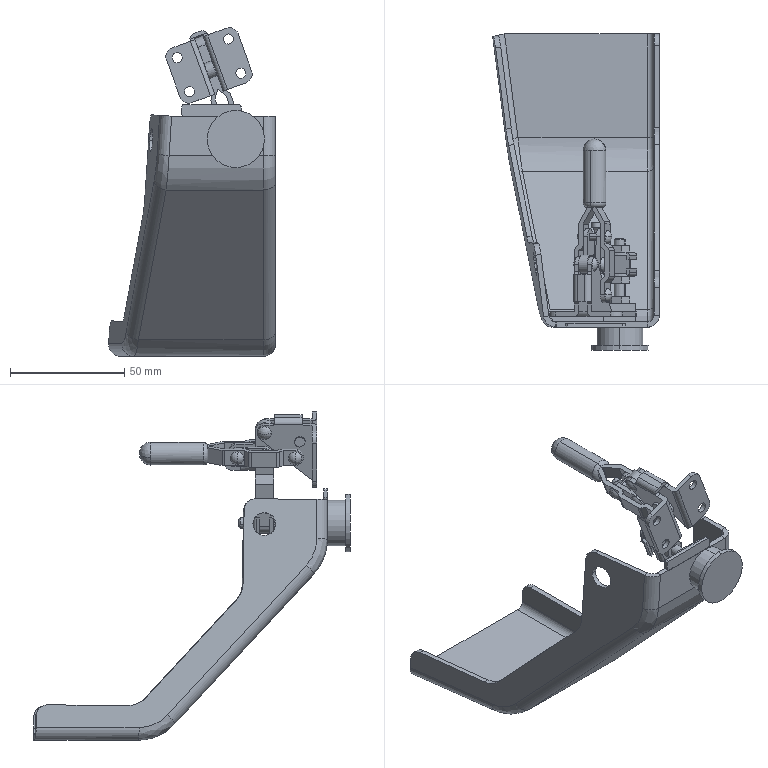Part | SolidWorks | 9 solids | 401 faces | box 72.927 x 138.4 x 143.686 mm | volume 52890 mm3 | plane 180 | cylinder 146 | cone 45 | sphere 18 | spline 6 | torus 6 | commonest cylinder face diameters 3 x26 10 x12 2 x10 7 x10 4 x9 4.4 x8